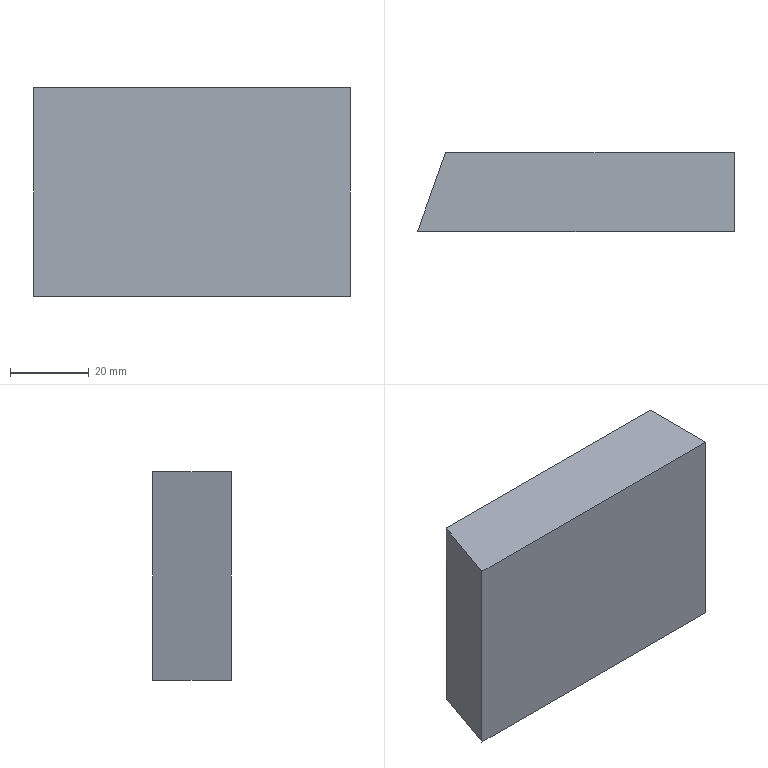Part | SolidWorks | features Extrusion 1 | 1 solid | 6 faces | box 80.4 x 20 x 53 mm | volume 81461 mm3 | plane 6
STEP:
#1=CARTESIAN_POINT('',(-80.4,0.,-26.5));
#2=VERTEX_POINT('',#1);
#3=CARTESIAN_POINT('',(0.,0.,-26.5));
#4=VERTEX_POINT('',#3);
#5=CARTESIAN_POINT('',(-80.4,0.,-26.5));
#6=DIRECTION('',(1.,0.,0.));
#7=VECTOR('',#6,1000.);
#8=LINE('',#5,#7);
#9=EDGE_CURVE('',#2,#4,#8,.T.);
#10=ORIENTED_EDGE('',*,*,#9,.T.);
#11=CARTESIAN_POINT('',(0.,0.,26.5));
#12=VERTEX_POINT('',#11);
#13=CARTESIAN_POINT('',(0.,0.,26.5));
#14=DIRECTION('',(0.,0.,-1.));
#15=VECTOR('',#14,1000.);
#16=LINE('',#13,#15);
#17=EDGE_CURVE('',#12,#4,#16,.T.);
#18=ORIENTED_EDGE('',*,*,#17,.F.);
#19=CARTESIAN_POINT('',(-80.4,0.,26.5));
#20=VERTEX_POINT('',#19);
#21=CARTESIAN_POINT('',(-80.4,0.,26.5));
#22=DIRECTION('',(1.,0.,0.));
#23=VECTOR('',#22,1000.);
#24=LINE('',#21,#23);
#25=EDGE_CURVE('',#20,#12,#24,.T.);
#26=ORIENTED_EDGE('',*,*,#25,.F.);
#27=CARTESIAN_POINT('',(-80.4,0.,26.5));
#28=DIRECTION('',(0.,0.,-1.));
#29=VECTOR('',#28,1000.);
#30=LINE('',#27,#29);
#31=EDGE_CURVE('',#20,#2,#30,.T.);
#32=ORIENTED_EDGE('',*,*,#31,.T.);
#33=EDGE_LOOP('',(#10,#18,#26,#32));
#34=FACE_OUTER_BOUND('',#33,.T.);
#35=CARTESIAN_POINT('',(-80.4,0.,26.5));
#36=DIRECTION('',(0.,1.,0.));
#37=DIRECTION('',(0.,0.,1.));
#38=AXIS2_PLACEMENT_3D('',#35,#36,#37);
#39=PLANE('',#38);
#40=ADVANCED_FACE('',(#34),#39,.F.);
#41=CARTESIAN_POINT('',(0.,20.,-26.5));
#42=VERTEX_POINT('',#41);
#43=CARTESIAN_POINT('',(0.,0.,-26.5));
#44=DIRECTION('',(0.,1.,0.));
#45=VECTOR('',#44,1000.);
#46=LINE('',#43,#45);
#47=EDGE_CURVE('',#4,#42,#46,.T.);
#48=ORIENTED_EDGE('',*,*,#47,.T.);
#49=CARTESIAN_POINT('',(0.,20.,26.5));
#50=VERTEX_POINT('',#49);
#51=CARTESIAN_POINT('',(0.,20.,26.5));
#52=DIRECTION('',(0.,0.,-1.));
#53=VECTOR('',#52,1000.);
#54=LINE('',#51,#53);
#55=EDGE_CURVE('',#50,#42,#54,.T.);
#56=ORIENTED_EDGE('',*,*,#55,.F.);
#57=CARTESIAN_POINT('',(0.,0.,26.5));
#58=DIRECTION('',(0.,1.,0.));
#59=VECTOR('',#58,1000.);
#60=LINE('',#57,#59);
#61=EDGE_CURVE('',#12,#50,#60,.T.);
#62=ORIENTED_EDGE('',*,*,#61,.F.);
#63=ORIENTED_EDGE('',*,*,#17,.T.);
#64=EDGE_LOOP('',(#48,#56,#62,#63));
#65=FACE_OUTER_BOUND('',#64,.T.);
#66=CARTESIAN_POINT('',(0.,0.,26.5));
#67=DIRECTION('',(-1.,0.,0.));
#68=DIRECTION('',(0.,0.,1.));
#69=AXIS2_PLACEMENT_3D('',#66,#67,#68);
#70=PLANE('',#69);
#71=ADVANCED_FACE('',(#65),#70,.F.);
#72=CARTESIAN_POINT('',(-73.3,20.,-26.5));
#73=VERTEX_POINT('',#72);
#74=CARTESIAN_POINT('',(0.,20.,-26.5));
#75=DIRECTION('',(-1.,0.,0.));
#76=VECTOR('',#75,1000.);
#77=LINE('',#74,#76);
#78=EDGE_CURVE('',#42,#73,#77,.T.);
#79=ORIENTED_EDGE('',*,*,#78,.T.);
#80=CARTESIAN_POINT('',(-73.3,20.,26.5));
#81=VERTEX_POINT('',#80);
#82=CARTESIAN_POINT('',(-73.3,20.,26.5));
#83=DIRECTION('',(0.,0.,-1.));
#84=VECTOR('',#83,1000.);
#85=LINE('',#82,#84);
#86=EDGE_CURVE('',#81,#73,#85,.T.);
#87=ORIENTED_EDGE('',*,*,#86,.F.);
#88=CARTESIAN_POINT('',(0.,20.,26.5));
#89=DIRECTION('',(-1.,0.,0.));
#90=VECTOR('',#89,1000.);
#91=LINE('',#88,#90);
#92=EDGE_CURVE('',#50,#81,#91,.T.);
#93=ORIENTED_EDGE('',*,*,#92,.F.);
#94=ORIENTED_EDGE('',*,*,#55,.T.);
#95=EDGE_LOOP('',(#79,#87,#93,#94));
#96=FACE_OUTER_BOUND('',#95,.T.);
#97=CARTESIAN_POINT('',(0.,20.,26.5));
#98=DIRECTION('',(0.,-1.,0.));
#99=DIRECTION('',(1.,0.,0.));
#100=AXIS2_PLACEMENT_3D('',#97,#98,#99);
#101=PLANE('',#100);
#102=ADVANCED_FACE('',(#96),#101,.F.);
#103=CARTESIAN_POINT('',(-73.3,20.,-26.5));
#104=DIRECTION('',(-0.3345,-0.9424,0.));
#105=VECTOR('',#104,1000.);
#106=LINE('',#103,#105);
#107=EDGE_CURVE('',#73,#2,#106,.T.);
#108=ORIENTED_EDGE('',*,*,#107,.T.);
#109=ORIENTED_EDGE('',*,*,#31,.F.);
#110=CARTESIAN_POINT('',(-73.3,20.,26.5));
#111=DIRECTION('',(-0.3345,-0.9424,0.));
#112=VECTOR('',#111,1000.);
#113=LINE('',#110,#112);
#114=EDGE_CURVE('',#81,#20,#113,.T.);
#115=ORIENTED_EDGE('',*,*,#114,.F.);
#116=ORIENTED_EDGE('',*,*,#86,.T.);
#117=EDGE_LOOP('',(#108,#109,#115,#116));
#118=FACE_OUTER_BOUND('',#117,.T.);
#119=CARTESIAN_POINT('',(-73.3,20.,26.5));
#120=DIRECTION('',(0.9424,-0.3345,0.));
#121=DIRECTION('',(0.3345,0.9424,0.));
#122=AXIS2_PLACEMENT_3D('',#119,#120,#121);
#123=PLANE('',#122);
#124=ADVANCED_FACE('',(#118),#123,.F.);
#125=ORIENTED_EDGE('',*,*,#25,.T.);
#126=ORIENTED_EDGE('',*,*,#61,.T.);
#127=ORIENTED_EDGE('',*,*,#92,.T.);
#128=ORIENTED_EDGE('',*,*,#114,.T.);
#129=EDGE_LOOP('',(#125,#126,#127,#128));
#130=FACE_OUTER_BOUND('',#129,.T.);
#131=CARTESIAN_POINT('',(0.,0.,26.5));
#132=DIRECTION('',(0.,0.,1.));
#133=DIRECTION('',(1.,0.,0.));
#134=AXIS2_PLACEMENT_3D('',#131,#132,#133);
#135=PLANE('',#134);
#136=ADVANCED_FACE('',(#130),#135,.T.);
#137=ORIENTED_EDGE('',*,*,#9,.F.);
#138=ORIENTED_EDGE('',*,*,#107,.F.);
#139=ORIENTED_EDGE('',*,*,#78,.F.);
#140=ORIENTED_EDGE('',*,*,#47,.F.);
#141=EDGE_LOOP('',(#137,#138,#139,#140));
#142=FACE_OUTER_BOUND('',#141,.T.);
#143=CARTESIAN_POINT('',(0.,0.,-26.5));
#144=DIRECTION('',(0.,0.,1.));
#145=DIRECTION('',(1.,0.,0.));
#146=AXIS2_PLACEMENT_3D('',#143,#144,#145);
#147=PLANE('',#146);
#148=ADVANCED_FACE('',(#142),#147,.F.);
#149=CLOSED_SHELL('',(#40,#71,#102,#124,#136,#148));
#150=MANIFOLD_SOLID_BREP('',#149);
#151=CARTESIAN_POINT('',(0.,0.,0.));
#152=DIRECTION('',(0.,0.,1.));
#153=DIRECTION('',(1.,0.,0.));
#154=AXIS2_PLACEMENT_3D('',#151,#152,#153);
#155=(LENGTH_UNIT()NAMED_UNIT(*)SI_UNIT(.MILLI.,.METRE.));
#156=UNCERTAINTY_MEASURE_WITH_UNIT(LENGTH_MEASURE(0.00001),#155,'','');
#157=(NAMED_UNIT(*)PLANE_ANGLE_UNIT()SI_UNIT($,.RADIAN.));
#158=(NAMED_UNIT(*)SI_UNIT($,.STERADIAN.)SOLID_ANGLE_UNIT());
#159=(GEOMETRIC_REPRESENTATION_CONTEXT(3)GLOBAL_UNCERTAINTY_ASSIGNED_CONTEXT((#156))GLOBAL_UNIT_ASSIGNED_CONTEXT((#155,#157,#158))REPRESENTATION_CONTEXT('',''));
#160=ADVANCED_BREP_SHAPE_REPRESENTATION('',(#150,#154),#159);